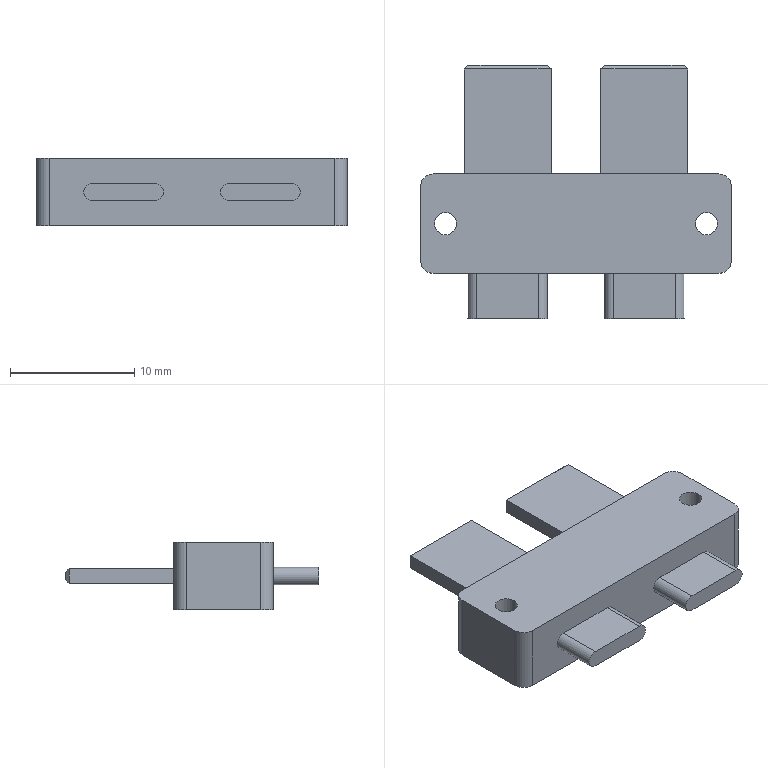Part | SolidWorks | features ICE 2, Chamfer 1, Extrusion 1, Fillet 1 | 1 solid | 42 faces | box 25 x 20.4 x 5.4 mm | volume 1256 mm3 | plane 30 | cylinder 12 | commonest cylinder face diameters 1.4 x4 1.8 x4 2 x4
STEP:
#1=CARTESIAN_POINT('',(-11.4,0.,5.4));
#2=VERTEX_POINT('',#1);
#3=CARTESIAN_POINT('',(-9.6,0.,5.4));
#4=VERTEX_POINT('',#3);
#5=CARTESIAN_POINT('',(-10.5,0.,5.4));
#6=DIRECTION('',(0.,0.,1.));
#7=DIRECTION('',(-1.,0.,0.));
#8=AXIS2_PLACEMENT_3D('',#5,#6,#7);
#9=CIRCLE('',#8,0.9);
#10=EDGE_CURVE('',#2,#4,#9,.T.);
#11=ORIENTED_EDGE('',*,*,#10,.T.);
#12=CARTESIAN_POINT('',(-9.6,0.,0.));
#13=VERTEX_POINT('',#12);
#14=CARTESIAN_POINT('',(-9.6,0.,5.4));
#15=DIRECTION('',(0.,0.,-1.));
#16=VECTOR('',#15,1000.);
#17=LINE('',#14,#16);
#18=EDGE_CURVE('',#4,#13,#17,.T.);
#19=ORIENTED_EDGE('',*,*,#18,.T.);
#20=CARTESIAN_POINT('',(-11.4,0.,0.));
#21=VERTEX_POINT('',#20);
#22=CARTESIAN_POINT('',(-10.5,0.,0.));
#23=DIRECTION('',(0.,0.,1.));
#24=DIRECTION('',(-1.,0.,0.));
#25=AXIS2_PLACEMENT_3D('',#22,#23,#24);
#26=CIRCLE('',#25,0.9);
#27=EDGE_CURVE('',#21,#13,#26,.T.);
#28=ORIENTED_EDGE('',*,*,#27,.F.);
#29=CARTESIAN_POINT('',(-11.4,0.,5.4));
#30=DIRECTION('',(0.,0.,-1.));
#31=VECTOR('',#30,1000.);
#32=LINE('',#29,#31);
#33=EDGE_CURVE('',#2,#21,#32,.T.);
#34=ORIENTED_EDGE('',*,*,#33,.F.);
#35=EDGE_LOOP('',(#11,#19,#28,#34));
#36=FACE_OUTER_BOUND('',#35,.T.);
#37=CARTESIAN_POINT('',(-10.5,0.,5.4));
#38=DIRECTION('',(0.,0.,-1.));
#39=DIRECTION('',(-1.,0.,0.));
#40=AXIS2_PLACEMENT_3D('',#37,#38,#39);
#41=CYLINDRICAL_SURFACE('',#40,0.9);
#42=ADVANCED_FACE('',(#36),#41,.F.);
#43=CARTESIAN_POINT('',(9.6,0.,5.4));
#44=VERTEX_POINT('',#43);
#45=CARTESIAN_POINT('',(11.4,0.,5.4));
#46=VERTEX_POINT('',#45);
#47=CARTESIAN_POINT('',(10.5,0.,5.4));
#48=DIRECTION('',(0.,0.,1.));
#49=DIRECTION('',(1.,0.,0.));
#50=AXIS2_PLACEMENT_3D('',#47,#48,#49);
#51=CIRCLE('',#50,0.9);
#52=EDGE_CURVE('',#44,#46,#51,.T.);
#53=ORIENTED_EDGE('',*,*,#52,.T.);
#54=CARTESIAN_POINT('',(11.4,0.,0.));
#55=VERTEX_POINT('',#54);
#56=CARTESIAN_POINT('',(11.4,0.,5.4));
#57=DIRECTION('',(0.,0.,-1.));
#58=VECTOR('',#57,1000.);
#59=LINE('',#56,#58);
#60=EDGE_CURVE('',#46,#55,#59,.T.);
#61=ORIENTED_EDGE('',*,*,#60,.T.);
#62=CARTESIAN_POINT('',(9.6,0.,0.));
#63=VERTEX_POINT('',#62);
#64=CARTESIAN_POINT('',(10.5,0.,0.));
#65=DIRECTION('',(0.,0.,1.));
#66=DIRECTION('',(1.,0.,0.));
#67=AXIS2_PLACEMENT_3D('',#64,#65,#66);
#68=CIRCLE('',#67,0.9);
#69=EDGE_CURVE('',#63,#55,#68,.T.);
#70=ORIENTED_EDGE('',*,*,#69,.F.);
#71=CARTESIAN_POINT('',(9.6,0.,5.4));
#72=DIRECTION('',(0.,0.,-1.));
#73=VECTOR('',#72,1000.);
#74=LINE('',#71,#73);
#75=EDGE_CURVE('',#44,#63,#74,.T.);
#76=ORIENTED_EDGE('',*,*,#75,.F.);
#77=EDGE_LOOP('',(#53,#61,#70,#76));
#78=FACE_OUTER_BOUND('',#77,.T.);
#79=CARTESIAN_POINT('',(10.5,0.,5.4));
#80=DIRECTION('',(0.,0.,-1.));
#81=DIRECTION('',(-1.,0.,0.));
#82=AXIS2_PLACEMENT_3D('',#79,#80,#81);
#83=CYLINDRICAL_SURFACE('',#82,0.9);
#84=ADVANCED_FACE('',(#78),#83,.F.);
#85=CARTESIAN_POINT('',(9.,4.,3.3));
#86=VERTEX_POINT('',#85);
#87=CARTESIAN_POINT('',(9.,4.,2.1));
#88=VERTEX_POINT('',#87);
#89=CARTESIAN_POINT('',(9.,4.,2.1));
#90=DIRECTION('',(0.,0.,-1.));
#91=VECTOR('',#90,1000.);
#92=LINE('',#89,#91);
#93=EDGE_CURVE('',#86,#88,#92,.T.);
#94=ORIENTED_EDGE('',*,*,#93,.F.);
#95=CARTESIAN_POINT('',(2.,4.,3.3));
#96=VERTEX_POINT('',#95);
#97=CARTESIAN_POINT('',(2.,4.,3.3));
#98=DIRECTION('',(1.,0.,0.));
#99=VECTOR('',#98,1000.);
#100=LINE('',#97,#99);
#101=EDGE_CURVE('',#96,#86,#100,.T.);
#102=ORIENTED_EDGE('',*,*,#101,.F.);
#103=CARTESIAN_POINT('',(2.,4.,2.1));
#104=VERTEX_POINT('',#103);
#105=CARTESIAN_POINT('',(2.,4.,2.1));
#106=DIRECTION('',(0.,0.,1.));
#107=VECTOR('',#106,1000.);
#108=LINE('',#105,#107);
#109=EDGE_CURVE('',#104,#96,#108,.T.);
#110=ORIENTED_EDGE('',*,*,#109,.F.);
#111=CARTESIAN_POINT('',(2.,4.,2.1));
#112=DIRECTION('',(-1.,0.,0.));
#113=VECTOR('',#112,1000.);
#114=LINE('',#111,#113);
#115=EDGE_CURVE('',#88,#104,#114,.T.);
#116=ORIENTED_EDGE('',*,*,#115,.F.);
#117=EDGE_LOOP('',(#94,#102,#110,#116));
#118=FACE_BOUND('',#117,.T.);
#119=CARTESIAN_POINT('',(11.5,4.,5.4));
#120=VERTEX_POINT('',#119);
#121=CARTESIAN_POINT('',(-11.5,4.,5.4));
#122=VERTEX_POINT('',#121);
#123=CARTESIAN_POINT('',(-12.5,4.,5.4));
#124=DIRECTION('',(-1.,0.,0.));
#125=VECTOR('',#124,1000.);
#126=LINE('',#123,#125);
#127=EDGE_CURVE('',#120,#122,#126,.T.);
#128=ORIENTED_EDGE('',*,*,#127,.F.);
#129=CARTESIAN_POINT('',(11.5,4.,0.));
#130=VERTEX_POINT('',#129);
#131=CARTESIAN_POINT('',(11.5,4.,5.4));
#132=DIRECTION('',(0.,0.,-1.));
#133=VECTOR('',#132,1000.);
#134=LINE('',#131,#133);
#135=EDGE_CURVE('',#120,#130,#134,.T.);
#136=ORIENTED_EDGE('',*,*,#135,.T.);
#137=CARTESIAN_POINT('',(-11.5,4.,0.));
#138=VERTEX_POINT('',#137);
#139=CARTESIAN_POINT('',(-12.5,4.,0.));
#140=DIRECTION('',(-1.,0.,0.));
#141=VECTOR('',#140,1000.);
#142=LINE('',#139,#141);
#143=EDGE_CURVE('',#130,#138,#142,.T.);
#144=ORIENTED_EDGE('',*,*,#143,.T.);
#145=CARTESIAN_POINT('',(-11.5,4.,5.4));
#146=DIRECTION('',(0.,0.,1.));
#147=VECTOR('',#146,1000.);
#148=LINE('',#145,#147);
#149=EDGE_CURVE('',#138,#122,#148,.T.);
#150=ORIENTED_EDGE('',*,*,#149,.T.);
#151=EDGE_LOOP('',(#128,#136,#144,#150));
#152=FACE_OUTER_BOUND('',#151,.T.);
#153=CARTESIAN_POINT('',(-2.,4.,3.3));
#154=VERTEX_POINT('',#153);
#155=CARTESIAN_POINT('',(-2.,4.,2.1));
#156=VERTEX_POINT('',#155);
#157=CARTESIAN_POINT('',(-2.,4.,2.1));
#158=DIRECTION('',(0.,0.,-1.));
#159=VECTOR('',#158,1000.);
#160=LINE('',#157,#159);
#161=EDGE_CURVE('',#154,#156,#160,.T.);
#162=ORIENTED_EDGE('',*,*,#161,.F.);
#163=CARTESIAN_POINT('',(-9.,4.,3.3));
#164=VERTEX_POINT('',#163);
#165=CARTESIAN_POINT('',(-2.,4.,3.3));
#166=DIRECTION('',(1.,0.,0.));
#167=VECTOR('',#166,1000.);
#168=LINE('',#165,#167);
#169=EDGE_CURVE('',#164,#154,#168,.T.);
#170=ORIENTED_EDGE('',*,*,#169,.F.);
#171=CARTESIAN_POINT('',(-9.,4.,2.1));
#172=VERTEX_POINT('',#171);
#173=CARTESIAN_POINT('',(-9.,4.,2.1));
#174=DIRECTION('',(0.,0.,1.));
#175=VECTOR('',#174,1000.);
#176=LINE('',#173,#175);
#177=EDGE_CURVE('',#172,#164,#176,.T.);
#178=ORIENTED_EDGE('',*,*,#177,.F.);
#179=CARTESIAN_POINT('',(-2.,4.,2.1));
#180=DIRECTION('',(-1.,0.,0.));
#181=VECTOR('',#180,1000.);
#182=LINE('',#179,#181);
#183=EDGE_CURVE('',#156,#172,#182,.T.);
#184=ORIENTED_EDGE('',*,*,#183,.F.);
#185=EDGE_LOOP('',(#162,#170,#178,#184));
#186=FACE_BOUND('',#185,.T.);
#187=CARTESIAN_POINT('',(-12.5,4.,5.4));
#188=DIRECTION('',(0.,-1.,0.));
#189=DIRECTION('',(0.,0.,-1.));
#190=AXIS2_PLACEMENT_3D('',#187,#188,#189);
#191=PLANE('',#190);
#192=ADVANCED_FACE('',(#118,#152,#186),#191,.F.);
#193=CARTESIAN_POINT('',(3.,-4.,3.4));
#194=VERTEX_POINT('',#193);
#195=CARTESIAN_POINT('',(3.,-4.,2.));
#196=VERTEX_POINT('',#195);
#197=CARTESIAN_POINT('',(3.,-4.,2.7));
#198=DIRECTION('',(0.,-1.,0.));
#199=DIRECTION('',(0.,0.,-1.));
#200=AXIS2_PLACEMENT_3D('',#197,#198,#199);
#201=CIRCLE('',#200,0.7);
#202=EDGE_CURVE('',#194,#196,#201,.T.);
#203=ORIENTED_EDGE('',*,*,#202,.F.);
#204=CARTESIAN_POINT('',(8.,-4.,3.4));
#205=VERTEX_POINT('',#204);
#206=CARTESIAN_POINT('',(3.,-4.,3.4));
#207=DIRECTION('',(-1.,0.,0.));
#208=VECTOR('',#207,1000.);
#209=LINE('',#206,#208);
#210=EDGE_CURVE('',#205,#194,#209,.T.);
#211=ORIENTED_EDGE('',*,*,#210,.F.);
#212=CARTESIAN_POINT('',(8.,-4.,2.));
#213=VERTEX_POINT('',#212);
#214=CARTESIAN_POINT('',(8.,-4.,2.7));
#215=DIRECTION('',(0.,-1.,0.));
#216=DIRECTION('',(0.,0.,-1.));
#217=AXIS2_PLACEMENT_3D('',#214,#215,#216);
#218=CIRCLE('',#217,0.7);
#219=EDGE_CURVE('',#213,#205,#218,.T.);
#220=ORIENTED_EDGE('',*,*,#219,.F.);
#221=CARTESIAN_POINT('',(3.,-4.,2.));
#222=DIRECTION('',(1.,0.,0.));
#223=VECTOR('',#222,1000.);
#224=LINE('',#221,#223);
#225=EDGE_CURVE('',#196,#213,#224,.T.);
#226=ORIENTED_EDGE('',*,*,#225,.F.);
#227=EDGE_LOOP('',(#203,#211,#220,#226));
#228=FACE_BOUND('',#227,.T.);
#229=CARTESIAN_POINT('',(-11.5,-4.,0.));
#230=VERTEX_POINT('',#229);
#231=CARTESIAN_POINT('',(11.5,-4.,0.));
#232=VERTEX_POINT('',#231);
#233=CARTESIAN_POINT('',(-12.5,-4.,0.));
#234=DIRECTION('',(1.,0.,0.));
#235=VECTOR('',#234,1000.);
#236=LINE('',#233,#235);
#237=EDGE_CURVE('',#230,#232,#236,.T.);
#238=ORIENTED_EDGE('',*,*,#237,.T.);
#239=CARTESIAN_POINT('',(11.5,-4.,5.4));
#240=VERTEX_POINT('',#239);
#241=CARTESIAN_POINT('',(11.5,-4.,5.4));
#242=DIRECTION('',(0.,0.,1.));
#243=VECTOR('',#242,1000.);
#244=LINE('',#241,#243);
#245=EDGE_CURVE('',#232,#240,#244,.T.);
#246=ORIENTED_EDGE('',*,*,#245,.T.);
#247=CARTESIAN_POINT('',(-11.5,-4.,5.4));
#248=VERTEX_POINT('',#247);
#249=CARTESIAN_POINT('',(-12.5,-4.,5.4));
#250=DIRECTION('',(1.,0.,0.));
#251=VECTOR('',#250,1000.);
#252=LINE('',#249,#251);
#253=EDGE_CURVE('',#248,#240,#252,.T.);
#254=ORIENTED_EDGE('',*,*,#253,.F.);
#255=CARTESIAN_POINT('',(-11.5,-4.,5.4));
#256=DIRECTION('',(0.,0.,-1.));
#257=VECTOR('',#256,1000.);
#258=LINE('',#255,#257);
#259=EDGE_CURVE('',#248,#230,#258,.T.);
#260=ORIENTED_EDGE('',*,*,#259,.T.);
#261=EDGE_LOOP('',(#238,#246,#254,#260));
#262=FACE_OUTER_BOUND('',#261,.T.);
#263=CARTESIAN_POINT('',(-3.,-4.,2.));
#264=VERTEX_POINT('',#263);
#265=CARTESIAN_POINT('',(-3.,-4.,3.4));
#266=VERTEX_POINT('',#265);
#267=CARTESIAN_POINT('',(-3.,-4.,2.7));
#268=DIRECTION('',(0.,-1.,0.));
#269=DIRECTION('',(0.,0.,1.));
#270=AXIS2_PLACEMENT_3D('',#267,#268,#269);
#271=CIRCLE('',#270,0.7);
#272=EDGE_CURVE('',#264,#266,#271,.T.);
#273=ORIENTED_EDGE('',*,*,#272,.F.);
#274=CARTESIAN_POINT('',(-8.,-4.,2.));
#275=VERTEX_POINT('',#274);
#276=CARTESIAN_POINT('',(-3.,-4.,2.));
#277=DIRECTION('',(1.,0.,0.));
#278=VECTOR('',#277,1000.);
#279=LINE('',#276,#278);
#280=EDGE_CURVE('',#275,#264,#279,.T.);
#281=ORIENTED_EDGE('',*,*,#280,.F.);
#282=CARTESIAN_POINT('',(-8.,-4.,3.4));
#283=VERTEX_POINT('',#282);
#284=CARTESIAN_POINT('',(-8.,-4.,2.7));
#285=DIRECTION('',(0.,-1.,0.));
#286=DIRECTION('',(0.,0.,1.));
#287=AXIS2_PLACEMENT_3D('',#284,#285,#286);
#288=CIRCLE('',#287,0.7);
#289=EDGE_CURVE('',#283,#275,#288,.T.);
#290=ORIENTED_EDGE('',*,*,#289,.F.);
#291=CARTESIAN_POINT('',(-3.,-4.,3.4));
#292=DIRECTION('',(-1.,0.,0.));
#293=VECTOR('',#292,1000.);
#294=LINE('',#291,#293);
#295=EDGE_CURVE('',#266,#283,#294,.T.);
#296=ORIENTED_EDGE('',*,*,#295,.F.);
#297=EDGE_LOOP('',(#273,#281,#290,#296));
#298=FACE_BOUND('',#297,.T.);
#299=CARTESIAN_POINT('',(-12.5,-4.,5.4));
#300=DIRECTION('',(0.,1.,0.));
#301=DIRECTION('',(0.,0.,1.));
#302=AXIS2_PLACEMENT_3D('',#299,#300,#301);
#303=PLANE('',#302);
#304=ADVANCED_FACE('',(#228,#262,#298),#303,.F.);
#305=ORIENTED_EDGE('',*,*,#52,.F.);
#306=CARTESIAN_POINT('',(10.5,0.,5.4));
#307=DIRECTION('',(0.,0.,1.));
#308=DIRECTION('',(1.,0.,0.));
#309=AXIS2_PLACEMENT_3D('',#306,#307,#308);
#310=CIRCLE('',#309,0.9);
#311=EDGE_CURVE('',#46,#44,#310,.T.);
#312=ORIENTED_EDGE('',*,*,#311,.F.);
#313=EDGE_LOOP('',(#305,#312));
#314=FACE_BOUND('',#313,.T.);
#315=ORIENTED_EDGE('',*,*,#253,.T.);
#316=CARTESIAN_POINT('',(12.5,-3.,5.4));
#317=VERTEX_POINT('',#316);
#318=CARTESIAN_POINT('',(11.5,-3.,5.4));
#319=DIRECTION('',(0.,0.,1.));
#320=DIRECTION('',(1.,0.,0.));
#321=AXIS2_PLACEMENT_3D('',#318,#319,#320);
#322=CIRCLE('',#321,1.);
#323=EDGE_CURVE('',#240,#317,#322,.T.);
#324=ORIENTED_EDGE('',*,*,#323,.T.);
#325=CARTESIAN_POINT('',(12.5,3.,5.4));
#326=VERTEX_POINT('',#325);
#327=CARTESIAN_POINT('',(12.5,4.,5.4));
#328=DIRECTION('',(0.,1.,0.));
#329=VECTOR('',#328,1000.);
#330=LINE('',#327,#329);
#331=EDGE_CURVE('',#317,#326,#330,.T.);
#332=ORIENTED_EDGE('',*,*,#331,.T.);
#333=CARTESIAN_POINT('',(11.5,3.,5.4));
#334=DIRECTION('',(0.,0.,1.));
#335=DIRECTION('',(1.,0.,0.));
#336=AXIS2_PLACEMENT_3D('',#333,#334,#335);
#337=CIRCLE('',#336,1.);
#338=EDGE_CURVE('',#326,#120,#337,.T.);
#339=ORIENTED_EDGE('',*,*,#338,.T.);
#340=ORIENTED_EDGE('',*,*,#127,.T.);
#341=CARTESIAN_POINT('',(-12.5,3.,5.4));
#342=VERTEX_POINT('',#341);
#343=CARTESIAN_POINT('',(-11.5,3.,5.4));
#344=DIRECTION('',(0.,0.,1.));
#345=DIRECTION('',(1.,0.,0.));
#346=AXIS2_PLACEMENT_3D('',#343,#344,#345);
#347=CIRCLE('',#346,1.);
#348=EDGE_CURVE('',#122,#342,#347,.T.);
#349=ORIENTED_EDGE('',*,*,#348,.T.);
#350=CARTESIAN_POINT('',(-12.5,-3.,5.4));
#351=VERTEX_POINT('',#350);
#352=CARTESIAN_POINT('',(-12.5,4.,5.4));
#353=DIRECTION('',(0.,-1.,0.));
#354=VECTOR('',#353,1000.);
#355=LINE('',#352,#354);
#356=EDGE_CURVE('',#342,#351,#355,.T.);
#357=ORIENTED_EDGE('',*,*,#356,.T.);
#358=CARTESIAN_POINT('',(-11.5,-3.,5.4));
#359=DIRECTION('',(0.,0.,1.));
#360=DIRECTION('',(1.,0.,0.));
#361=AXIS2_PLACEMENT_3D('',#358,#359,#360);
#362=CIRCLE('',#361,1.);
#363=EDGE_CURVE('',#351,#248,#362,.T.);
#364=ORIENTED_EDGE('',*,*,#363,.T.);
#365=EDGE_LOOP('',(#315,#324,#332,#339,#340,#349,#357,#364));
#366=FACE_OUTER_BOUND('',#365,.T.);
#367=ORIENTED_EDGE('',*,*,#10,.F.);
#368=CARTESIAN_POINT('',(-10.5,0.,5.4));
#369=DIRECTION('',(0.,0.,1.));
#370=DIRECTION('',(-1.,0.,0.));
#371=AXIS2_PLACEMENT_3D('',#368,#369,#370);
#372=CIRCLE('',#371,0.9);
#373=EDGE_CURVE('',#4,#2,#372,.T.);
#374=ORIENTED_EDGE('',*,*,#373,.F.);
#375=EDGE_LOOP('',(#367,#374));
#376=FACE_BOUND('',#375,.T.);
#377=CARTESIAN_POINT('',(0.,0.,5.4));
#378=DIRECTION('',(0.,0.,1.));
#379=DIRECTION('',(1.,0.,0.));
#380=AXIS2_PLACEMENT_3D('',#377,#378,#379);
#381=PLANE('',#380);
#382=ADVANCED_FACE('',(#314,#366,#376),#381,.T.);
#383=CARTESIAN_POINT('',(12.5,-3.,0.));
#384=VERTEX_POINT('',#383);
#385=CARTESIAN_POINT('',(12.5,3.,0.));
#386=VERTEX_POINT('',#385);
#387=CARTESIAN_POINT('',(12.5,4.,0.));
#388=DIRECTION('',(0.,1.,0.));
#389=VECTOR('',#388,1000.);
#390=LINE('',#387,#389);
#391=EDGE_CURVE('',#384,#386,#390,.T.);
#392=ORIENTED_EDGE('',*,*,#391,.F.);
#393=CARTESIAN_POINT('',(11.5,-3.,0.));
#394=DIRECTION('',(0.,0.,-1.));
#395=DIRECTION('',(1.,0.,0.));
#396=AXIS2_PLACEMENT_3D('',#393,#394,#395);
#397=CIRCLE('',#396,1.);
#398=EDGE_CURVE('',#384,#232,#397,.T.);
#399=ORIENTED_EDGE('',*,*,#398,.T.);
#400=ORIENTED_EDGE('',*,*,#237,.F.);
#401=CARTESIAN_POINT('',(-12.5,-3.,0.));
#402=VERTEX_POINT('',#401);
#403=CARTESIAN_POINT('',(-11.5,-3.,0.));
#404=DIRECTION('',(0.,0.,-1.));
#405=DIRECTION('',(1.,0.,0.));
#406=AXIS2_PLACEMENT_3D('',#403,#404,#405);
#407=CIRCLE('',#406,1.);
#408=EDGE_CURVE('',#230,#402,#407,.T.);
#409=ORIENTED_EDGE('',*,*,#408,.T.);
#410=CARTESIAN_POINT('',(-12.5,3.,0.));
#411=VERTEX_POINT('',#410);
#412=CARTESIAN_POINT('',(-12.5,4.,0.));
#413=DIRECTION('',(0.,-1.,0.));
#414=VECTOR('',#413,1000.);
#415=LINE('',#412,#414);
#416=EDGE_CURVE('',#411,#402,#415,.T.);
#417=ORIENTED_EDGE('',*,*,#416,.F.);
#418=CARTESIAN_POINT('',(-11.5,3.,0.));
#419=DIRECTION('',(0.,0.,-1.));
#420=DIRECTION('',(1.,0.,0.));
#421=AXIS2_PLACEMENT_3D('',#418,#419,#420);
#422=CIRCLE('',#421,1.);
#423=EDGE_CURVE('',#411,#138,#422,.T.);
#424=ORIENTED_EDGE('',*,*,#423,.T.);
#425=ORIENTED_EDGE('',*,*,#143,.F.);
#426=CARTESIAN_POINT('',(11.5,3.,0.));
#427=DIRECTION('',(0.,0.,-1.));
#428=DIRECTION('',(1.,0.,0.));
#429=AXIS2_PLACEMENT_3D('',#426,#427,#428);
#430=CIRCLE('',#429,1.);
#431=EDGE_CURVE('',#130,#386,#430,.T.);
#432=ORIENTED_EDGE('',*,*,#431,.T.);
#433=EDGE_LOOP('',(#392,#399,#400,#409,#417,#424,#425,#432));
#434=FACE_OUTER_BOUND('',#433,.T.);
#435=ORIENTED_EDGE('',*,*,#69,.T.);
#436=CARTESIAN_POINT('',(10.5,0.,0.));
#437=DIRECTION('',(0.,0.,1.));
#438=DIRECTION('',(1.,0.,0.));
#439=AXIS2_PLACEMENT_3D('',#436,#437,#438);
#440=CIRCLE('',#439,0.9);
#441=EDGE_CURVE('',#55,#63,#440,.T.);
#442=ORIENTED_EDGE('',*,*,#441,.T.);
#443=EDGE_LOOP('',(#435,#442));
#444=FACE_BOUND('',#443,.T.);
#445=ORIENTED_EDGE('',*,*,#27,.T.);
#446=CARTESIAN_POINT('',(-10.5,0.,0.));
#447=DIRECTION('',(0.,0.,1.));
#448=DIRECTION('',(-1.,0.,0.));
#449=AXIS2_PLACEMENT_3D('',#446,#447,#448);
#450=CIRCLE('',#449,0.9);
#451=EDGE_CURVE('',#13,#21,#450,.T.);
#452=ORIENTED_EDGE('',*,*,#451,.T.);
#453=EDGE_LOOP('',(#445,#452));
#454=FACE_BOUND('',#453,.T.);
#455=CARTESIAN_POINT('',(0.,0.,0.));
#456=DIRECTION('',(0.,0.,1.));
#457=DIRECTION('',(1.,0.,0.));
#458=AXIS2_PLACEMENT_3D('',#455,#456,#457);
#459=PLANE('',#458);
#460=ADVANCED_FACE('',(#434,#444,#454),#459,.F.);
#461=ORIENTED_EDGE('',*,*,#331,.F.);
#462=CARTESIAN_POINT('',(12.5,-3.,5.4));
#463=DIRECTION('',(0.,0.,-1.));
#464=VECTOR('',#463,1000.);
#465=LINE('',#462,#464);
#466=EDGE_CURVE('',#317,#384,#465,.T.);
#467=ORIENTED_EDGE('',*,*,#466,.T.);
#468=ORIENTED_EDGE('',*,*,#391,.T.);
#469=CARTESIAN_POINT('',(12.5,3.,5.4));
#470=DIRECTION('',(0.,0.,1.));
#471=VECTOR('',#470,1000.);
#472=LINE('',#469,#471);
#473=EDGE_CURVE('',#386,#326,#472,.T.);
#474=ORIENTED_EDGE('',*,*,#473,.T.);
#475=EDGE_LOOP('',(#461,#467,#468,#474));
#476=FACE_OUTER_BOUND('',#475,.T.);
#477=CARTESIAN_POINT('',(12.5,4.,5.4));
#478=DIRECTION('',(-1.,0.,0.));
#479=DIRECTION('',(0.,0.,1.));
#480=AXIS2_PLACEMENT_3D('',#477,#478,#479);
#481=PLANE('',#480);
#482=ADVANCED_FACE('',(#476),#481,.F.);
#483=ORIENTED_EDGE('',*,*,#416,.T.);
#484=CARTESIAN_POINT('',(-12.5,-3.,5.4));
#485=DIRECTION('',(0.,0.,1.));
#486=VECTOR('',#485,1000.);
#487=LINE('',#484,#486);
#488=EDGE_CURVE('',#402,#351,#487,.T.);
#489=ORIENTED_EDGE('',*,*,#488,.T.);
#490=ORIENTED_EDGE('',*,*,#356,.F.);
#491=CARTESIAN_POINT('',(-12.5,3.,5.4));
#492=DIRECTION('',(0.,0.,-1.));
#493=VECTOR('',#492,1000.);
#494=LINE('',#491,#493);
#495=EDGE_CURVE('',#342,#411,#494,.T.);
#496=ORIENTED_EDGE('',*,*,#495,.T.);
#497=EDGE_LOOP('',(#483,#489,#490,#496));
#498=FACE_OUTER_BOUND('',#497,.T.);
#499=CARTESIAN_POINT('',(-12.5,4.,5.4));
#500=DIRECTION('',(1.,0.,0.));
#501=DIRECTION('',(0.,1.,0.));
#502=AXIS2_PLACEMENT_3D('',#499,#500,#501);
#503=PLANE('',#502);
#504=ADVANCED_FACE('',(#498),#503,.F.);
#505=ORIENTED_EDGE('',*,*,#60,.F.);
#506=ORIENTED_EDGE('',*,*,#311,.T.);
#507=ORIENTED_EDGE('',*,*,#75,.T.);
#508=ORIENTED_EDGE('',*,*,#441,.F.);
#509=EDGE_LOOP('',(#505,#506,#507,#508));
#510=FACE_OUTER_BOUND('',#509,.T.);
#511=CARTESIAN_POINT('',(10.5,0.,5.4));
#512=DIRECTION('',(0.,0.,-1.));
#513=DIRECTION('',(-1.,0.,0.));
#514=AXIS2_PLACEMENT_3D('',#511,#512,#513);
#515=CYLINDRICAL_SURFACE('',#514,0.9);
#516=ADVANCED_FACE('',(#510),#515,.F.);
#517=ORIENTED_EDGE('',*,*,#18,.F.);
#518=ORIENTED_EDGE('',*,*,#373,.T.);
#519=ORIENTED_EDGE('',*,*,#33,.T.);
#520=ORIENTED_EDGE('',*,*,#451,.F.);
#521=EDGE_LOOP('',(#517,#518,#519,#520));
#522=FACE_OUTER_BOUND('',#521,.T.);
#523=CARTESIAN_POINT('',(-10.5,0.,5.4));
#524=DIRECTION('',(0.,0.,-1.));
#525=DIRECTION('',(-1.,0.,0.));
#526=AXIS2_PLACEMENT_3D('',#523,#524,#525);
#527=CYLINDRICAL_SURFACE('',#526,0.9);
#528=ADVANCED_FACE('',(#522),#527,.F.);
#529=ORIENTED_EDGE('',*,*,#202,.T.);
#530=CARTESIAN_POINT('',(3.,-7.65,2.));
#531=VERTEX_POINT('',#530);
#532=CARTESIAN_POINT('',(3.,-7.65,2.));
#533=DIRECTION('',(0.,1.,0.));
#534=VECTOR('',#533,1000.);
#535=LINE('',#532,#534);
#536=EDGE_CURVE('',#531,#196,#535,.T.);
#537=ORIENTED_EDGE('',*,*,#536,.F.);
#538=CARTESIAN_POINT('',(3.,-7.65,3.4));
#539=VERTEX_POINT('',#538);
#540=CARTESIAN_POINT('',(3.,-7.65,2.7));
#541=DIRECTION('',(0.,-1.,0.));
#542=DIRECTION('',(0.,0.,-1.));
#543=AXIS2_PLACEMENT_3D('',#540,#541,#542);
#544=CIRCLE('',#543,0.7);
#545=EDGE_CURVE('',#539,#531,#544,.T.);
#546=ORIENTED_EDGE('',*,*,#545,.F.);
#547=CARTESIAN_POINT('',(3.,-7.65,3.4));
#548=DIRECTION('',(0.,1.,0.));
#549=VECTOR('',#548,1000.);
#550=LINE('',#547,#549);
#551=EDGE_CURVE('',#539,#194,#550,.T.);
#552=ORIENTED_EDGE('',*,*,#551,.T.);
#553=EDGE_LOOP('',(#529,#537,#546,#552));
#554=FACE_OUTER_BOUND('',#553,.T.);
#555=CARTESIAN_POINT('',(3.,-7.65,2.7));
#556=DIRECTION('',(0.,1.,0.));
#557=DIRECTION('',(0.,0.,1.));
#558=AXIS2_PLACEMENT_3D('',#555,#556,#557);
#559=CYLINDRICAL_SURFACE('',#558,0.7);
#560=ADVANCED_FACE('',(#554),#559,.T.);
#561=ORIENTED_EDGE('',*,*,#225,.T.);
#562=CARTESIAN_POINT('',(8.,-7.65,2.));
#563=VERTEX_POINT('',#562);
#564=CARTESIAN_POINT('',(8.,-7.65,2.));
#565=DIRECTION('',(0.,1.,0.));
#566=VECTOR('',#565,1000.);
#567=LINE('',#564,#566);
#568=EDGE_CURVE('',#563,#213,#567,.T.);
#569=ORIENTED_EDGE('',*,*,#568,.F.);
#570=CARTESIAN_POINT('',(3.,-7.65,2.));
#571=DIRECTION('',(1.,0.,0.));
#572=VECTOR('',#571,1000.);
#573=LINE('',#570,#572);
#574=EDGE_CURVE('',#531,#563,#573,.T.);
#575=ORIENTED_EDGE('',*,*,#574,.F.);
#576=ORIENTED_EDGE('',*,*,#536,.T.);
#577=EDGE_LOOP('',(#561,#569,#575,#576));
#578=FACE_OUTER_BOUND('',#577,.T.);
#579=CARTESIAN_POINT('',(3.,-7.65,2.));
#580=DIRECTION('',(0.,0.,1.));
#581=DIRECTION('',(1.,0.,0.));
#582=AXIS2_PLACEMENT_3D('',#579,#580,#581);
#583=PLANE('',#582);
#584=ADVANCED_FACE('',(#578),#583,.F.);
#585=ORIENTED_EDGE('',*,*,#219,.T.);
#586=CARTESIAN_POINT('',(8.,-7.65,3.4));
#587=VERTEX_POINT('',#586);
#588=CARTESIAN_POINT('',(8.,-7.65,3.4));
#589=DIRECTION('',(0.,1.,0.));
#590=VECTOR('',#589,1000.);
#591=LINE('',#588,#590);
#592=EDGE_CURVE('',#587,#205,#591,.T.);
#593=ORIENTED_EDGE('',*,*,#592,.F.);
#594=CARTESIAN_POINT('',(8.,-7.65,2.7));
#595=DIRECTION('',(0.,-1.,0.));
#596=DIRECTION('',(0.,0.,-1.));
#597=AXIS2_PLACEMENT_3D('',#594,#595,#596);
#598=CIRCLE('',#597,0.7);
#599=EDGE_CURVE('',#563,#587,#598,.T.);
#600=ORIENTED_EDGE('',*,*,#599,.F.);
#601=ORIENTED_EDGE('',*,*,#568,.T.);
#602=EDGE_LOOP('',(#585,#593,#600,#601));
#603=FACE_OUTER_BOUND('',#602,.T.);
#604=CARTESIAN_POINT('',(8.,-7.65,2.7));
#605=DIRECTION('',(0.,1.,0.));
#606=DIRECTION('',(0.,0.,1.));
#607=AXIS2_PLACEMENT_3D('',#604,#605,#606);
#608=CYLINDRICAL_SURFACE('',#607,0.7);
#609=ADVANCED_FACE('',(#603),#608,.T.);
#610=ORIENTED_EDGE('',*,*,#210,.T.);
#611=ORIENTED_EDGE('',*,*,#551,.F.);
#612=CARTESIAN_POINT('',(3.,-7.65,3.4));
#613=DIRECTION('',(-1.,0.,0.));
#614=VECTOR('',#613,1000.);
#615=LINE('',#612,#614);
#616=EDGE_CURVE('',#587,#539,#615,.T.);
#617=ORIENTED_EDGE('',*,*,#616,.F.);
#618=ORIENTED_EDGE('',*,*,#592,.T.);
#619=EDGE_LOOP('',(#610,#611,#617,#618));
#620=FACE_OUTER_BOUND('',#619,.T.);
#621=CARTESIAN_POINT('',(3.,-7.65,3.4));
#622=DIRECTION('',(0.,0.,-1.));
#623=DIRECTION('',(-1.,0.,0.));
#624=AXIS2_PLACEMENT_3D('',#621,#622,#623);
#625=PLANE('',#624);
#626=ADVANCED_FACE('',(#620),#625,.F.);
#627=ORIENTED_EDGE('',*,*,#545,.T.);
#628=ORIENTED_EDGE('',*,*,#574,.T.);
#629=ORIENTED_EDGE('',*,*,#599,.T.);
#630=ORIENTED_EDGE('',*,*,#616,.T.);
#631=EDGE_LOOP('',(#627,#628,#629,#630));
#632=FACE_OUTER_BOUND('',#631,.T.);
#633=CARTESIAN_POINT('',(3.,-7.65,2.7));
#634=DIRECTION('',(0.,-1.,0.));
#635=DIRECTION('',(0.,0.,-1.));
#636=AXIS2_PLACEMENT_3D('',#633,#634,#635);
#637=PLANE('',#636);
#638=ADVANCED_FACE('',(#632),#637,.T.);
#639=ORIENTED_EDGE('',*,*,#272,.T.);
#640=CARTESIAN_POINT('',(-3.,-7.65,3.4));
#641=VERTEX_POINT('',#640);
#642=CARTESIAN_POINT('',(-3.,-7.65,3.4));
#643=DIRECTION('',(0.,1.,0.));
#644=VECTOR('',#643,1000.);
#645=LINE('',#642,#644);
#646=EDGE_CURVE('',#641,#266,#645,.T.);
#647=ORIENTED_EDGE('',*,*,#646,.F.);
#648=CARTESIAN_POINT('',(-3.,-7.65,2.));
#649=VERTEX_POINT('',#648);
#650=CARTESIAN_POINT('',(-3.,-7.65,2.7));
#651=DIRECTION('',(0.,-1.,0.));
#652=DIRECTION('',(0.,0.,1.));
#653=AXIS2_PLACEMENT_3D('',#650,#651,#652);
#654=CIRCLE('',#653,0.7);
#655=EDGE_CURVE('',#649,#641,#654,.T.);
#656=ORIENTED_EDGE('',*,*,#655,.F.);
#657=CARTESIAN_POINT('',(-3.,-7.65,2.));
#658=DIRECTION('',(0.,1.,0.));
#659=VECTOR('',#658,1000.);
#660=LINE('',#657,#659);
#661=EDGE_CURVE('',#649,#264,#660,.T.);
#662=ORIENTED_EDGE('',*,*,#661,.T.);
#663=EDGE_LOOP('',(#639,#647,#656,#662));
#664=FACE_OUTER_BOUND('',#663,.T.);
#665=CARTESIAN_POINT('',(-3.,-7.65,2.7));
#666=DIRECTION('',(0.,1.,0.));
#667=DIRECTION('',(0.,0.,1.));
#668=AXIS2_PLACEMENT_3D('',#665,#666,#667);
#669=CYLINDRICAL_SURFACE('',#668,0.7);
#670=ADVANCED_FACE('',(#664),#669,.T.);
#671=ORIENTED_EDGE('',*,*,#295,.T.);
#672=CARTESIAN_POINT('',(-8.,-7.65,3.4));
#673=VERTEX_POINT('',#672);
#674=CARTESIAN_POINT('',(-8.,-7.65,3.4));
#675=DIRECTION('',(0.,1.,0.));
#676=VECTOR('',#675,1000.);
#677=LINE('',#674,#676);
#678=EDGE_CURVE('',#673,#283,#677,.T.);
#679=ORIENTED_EDGE('',*,*,#678,.F.);
#680=CARTESIAN_POINT('',(-3.,-7.65,3.4));
#681=DIRECTION('',(-1.,0.,0.));
#682=VECTOR('',#681,1000.);
#683=LINE('',#680,#682);
#684=EDGE_CURVE('',#641,#673,#683,.T.);
#685=ORIENTED_EDGE('',*,*,#684,.F.);
#686=ORIENTED_EDGE('',*,*,#646,.T.);
#687=EDGE_LOOP('',(#671,#679,#685,#686));
#688=FACE_OUTER_BOUND('',#687,.T.);
#689=CARTESIAN_POINT('',(-3.,-7.65,3.4));
#690=DIRECTION('',(0.,0.,-1.));
#691=DIRECTION('',(-1.,0.,0.));
#692=AXIS2_PLACEMENT_3D('',#689,#690,#691);
#693=PLANE('',#692);
#694=ADVANCED_FACE('',(#688),#693,.F.);
#695=ORIENTED_EDGE('',*,*,#289,.T.);
#696=CARTESIAN_POINT('',(-8.,-7.65,2.));
#697=VERTEX_POINT('',#696);
#698=CARTESIAN_POINT('',(-8.,-7.65,2.));
#699=DIRECTION('',(0.,1.,0.));
#700=VECTOR('',#699,1000.);
#701=LINE('',#698,#700);
#702=EDGE_CURVE('',#697,#275,#701,.T.);
#703=ORIENTED_EDGE('',*,*,#702,.F.);
#704=CARTESIAN_POINT('',(-8.,-7.65,2.7));
#705=DIRECTION('',(0.,-1.,0.));
#706=DIRECTION('',(0.,0.,1.));
#707=AXIS2_PLACEMENT_3D('',#704,#705,#706);
#708=CIRCLE('',#707,0.7);
#709=EDGE_CURVE('',#673,#697,#708,.T.);
#710=ORIENTED_EDGE('',*,*,#709,.F.);
#711=ORIENTED_EDGE('',*,*,#678,.T.);
#712=EDGE_LOOP('',(#695,#703,#710,#711));
#713=FACE_OUTER_BOUND('',#712,.T.);
#714=CARTESIAN_POINT('',(-8.,-7.65,2.7));
#715=DIRECTION('',(0.,1.,0.));
#716=DIRECTION('',(0.,0.,1.));
#717=AXIS2_PLACEMENT_3D('',#714,#715,#716);
#718=CYLINDRICAL_SURFACE('',#717,0.7);
#719=ADVANCED_FACE('',(#713),#718,.T.);
#720=ORIENTED_EDGE('',*,*,#280,.T.);
#721=ORIENTED_EDGE('',*,*,#661,.F.);
#722=CARTESIAN_POINT('',(-3.,-7.65,2.));
#723=DIRECTION('',(1.,0.,0.));
#724=VECTOR('',#723,1000.);
#725=LINE('',#722,#724);
#726=EDGE_CURVE('',#697,#649,#725,.T.);
#727=ORIENTED_EDGE('',*,*,#726,.F.);
#728=ORIENTED_EDGE('',*,*,#702,.T.);
#729=EDGE_LOOP('',(#720,#721,#727,#728));
#730=FACE_OUTER_BOUND('',#729,.T.);
#731=CARTESIAN_POINT('',(-3.,-7.65,2.));
#732=DIRECTION('',(0.,0.,1.));
#733=DIRECTION('',(1.,0.,0.));
#734=AXIS2_PLACEMENT_3D('',#731,#732,#733);
#735=PLANE('',#734);
#736=ADVANCED_FACE('',(#730),#735,.F.);
#737=ORIENTED_EDGE('',*,*,#655,.T.);
#738=ORIENTED_EDGE('',*,*,#684,.T.);
#739=ORIENTED_EDGE('',*,*,#709,.T.);
#740=ORIENTED_EDGE('',*,*,#726,.T.);
#741=EDGE_LOOP('',(#737,#738,#739,#740));
#742=FACE_OUTER_BOUND('',#741,.T.);
#743=CARTESIAN_POINT('',(-3.,-7.65,2.7));
#744=DIRECTION('',(0.,1.,0.));
#745=DIRECTION('',(0.,0.,1.));
#746=AXIS2_PLACEMENT_3D('',#743,#744,#745);
#747=PLANE('',#746);
#748=ADVANCED_FACE('',(#742),#747,.F.);
#749=CARTESIAN_POINT('',(9.,12.45,2.1));
#750=VERTEX_POINT('',#749);
#751=CARTESIAN_POINT('',(9.,12.75,2.1));
#752=DIRECTION('',(0.,-1.,0.));
#753=VECTOR('',#752,1000.);
#754=LINE('',#751,#753);
#755=EDGE_CURVE('',#750,#88,#754,.T.);
#756=ORIENTED_EDGE('',*,*,#755,.F.);
#757=CARTESIAN_POINT('',(9.,12.45,3.3));
#758=VERTEX_POINT('',#757);
#759=CARTESIAN_POINT('',(9.,12.45,3.3));
#760=DIRECTION('',(0.,0.,1.));
#761=VECTOR('',#760,1000.);
#762=LINE('',#759,#761);
#763=EDGE_CURVE('',#750,#758,#762,.T.);
#764=ORIENTED_EDGE('',*,*,#763,.T.);
#765=CARTESIAN_POINT('',(9.,12.75,3.3));
#766=DIRECTION('',(0.,-1.,0.));
#767=VECTOR('',#766,1000.);
#768=LINE('',#765,#767);
#769=EDGE_CURVE('',#758,#86,#768,.T.);
#770=ORIENTED_EDGE('',*,*,#769,.T.);
#771=ORIENTED_EDGE('',*,*,#93,.T.);
#772=EDGE_LOOP('',(#756,#764,#770,#771));
#773=FACE_OUTER_BOUND('',#772,.T.);
#774=CARTESIAN_POINT('',(9.,12.75,2.1));
#775=DIRECTION('',(-1.,0.,0.));
#776=DIRECTION('',(0.,0.,1.));
#777=AXIS2_PLACEMENT_3D('',#774,#775,#776);
#778=PLANE('',#777);
#779=ADVANCED_FACE('',(#773),#778,.F.);
#780=CARTESIAN_POINT('',(2.,12.45,2.1));
#781=VERTEX_POINT('',#780);
#782=CARTESIAN_POINT('',(2.,12.75,2.1));
#783=DIRECTION('',(0.,-1.,0.));
#784=VECTOR('',#783,1000.);
#785=LINE('',#782,#784);
#786=EDGE_CURVE('',#781,#104,#785,.T.);
#787=ORIENTED_EDGE('',*,*,#786,.F.);
#788=CARTESIAN_POINT('',(9.,12.45,2.1));
#789=DIRECTION('',(1.,0.,0.));
#790=VECTOR('',#789,1000.);
#791=LINE('',#788,#790);
#792=EDGE_CURVE('',#781,#750,#791,.T.);
#793=ORIENTED_EDGE('',*,*,#792,.T.);
#794=ORIENTED_EDGE('',*,*,#755,.T.);
#795=ORIENTED_EDGE('',*,*,#115,.T.);
#796=EDGE_LOOP('',(#787,#793,#794,#795));
#797=FACE_OUTER_BOUND('',#796,.T.);
#798=CARTESIAN_POINT('',(2.,12.75,2.1));
#799=DIRECTION('',(0.,0.,1.));
#800=DIRECTION('',(1.,0.,0.));
#801=AXIS2_PLACEMENT_3D('',#798,#799,#800);
#802=PLANE('',#801);
#803=ADVANCED_FACE('',(#797),#802,.F.);
#804=CARTESIAN_POINT('',(2.,12.45,3.3));
#805=VERTEX_POINT('',#804);
#806=CARTESIAN_POINT('',(2.,12.75,3.3));
#807=DIRECTION('',(0.,-1.,0.));
#808=VECTOR('',#807,1000.);
#809=LINE('',#806,#808);
#810=EDGE_CURVE('',#805,#96,#809,.T.);
#811=ORIENTED_EDGE('',*,*,#810,.F.);
#812=CARTESIAN_POINT('',(2.,12.45,2.1));
#813=DIRECTION('',(0.,0.,-1.));
#814=VECTOR('',#813,1000.);
#815=LINE('',#812,#814);
#816=EDGE_CURVE('',#805,#781,#815,.T.);
#817=ORIENTED_EDGE('',*,*,#816,.T.);
#818=ORIENTED_EDGE('',*,*,#786,.T.);
#819=ORIENTED_EDGE('',*,*,#109,.T.);
#820=EDGE_LOOP('',(#811,#817,#818,#819));
#821=FACE_OUTER_BOUND('',#820,.T.);
#822=CARTESIAN_POINT('',(2.,12.75,2.1));
#823=DIRECTION('',(1.,0.,0.));
#824=DIRECTION('',(0.,0.,-1.));
#825=AXIS2_PLACEMENT_3D('',#822,#823,#824);
#826=PLANE('',#825);
#827=ADVANCED_FACE('',(#821),#826,.F.);
#828=ORIENTED_EDGE('',*,*,#769,.F.);
#829=CARTESIAN_POINT('',(2.,12.45,3.3));
#830=DIRECTION('',(-1.,0.,0.));
#831=VECTOR('',#830,1000.);
#832=LINE('',#829,#831);
#833=EDGE_CURVE('',#758,#805,#832,.T.);
#834=ORIENTED_EDGE('',*,*,#833,.T.);
#835=ORIENTED_EDGE('',*,*,#810,.T.);
#836=ORIENTED_EDGE('',*,*,#101,.T.);
#837=EDGE_LOOP('',(#828,#834,#835,#836));
#838=FACE_OUTER_BOUND('',#837,.T.);
#839=CARTESIAN_POINT('',(2.,12.75,3.3));
#840=DIRECTION('',(0.,0.,-1.));
#841=DIRECTION('',(-1.,0.,0.));
#842=AXIS2_PLACEMENT_3D('',#839,#840,#841);
#843=PLANE('',#842);
#844=ADVANCED_FACE('',(#838),#843,.F.);
#845=CARTESIAN_POINT('',(2.3,12.75,2.4));
#846=VERTEX_POINT('',#845);
#847=CARTESIAN_POINT('',(2.3,12.75,3.));
#848=VERTEX_POINT('',#847);
#849=CARTESIAN_POINT('',(2.3,12.75,3.3));
#850=DIRECTION('',(0.,0.,1.));
#851=VECTOR('',#850,1000.);
#852=LINE('',#849,#851);
#853=EDGE_CURVE('',#846,#848,#852,.T.);
#854=ORIENTED_EDGE('',*,*,#853,.T.);
#855=CARTESIAN_POINT('',(8.7,12.75,3.));
#856=VERTEX_POINT('',#855);
#857=CARTESIAN_POINT('',(9.,12.75,3.));
#858=DIRECTION('',(1.,0.,0.));
#859=VECTOR('',#858,1000.);
#860=LINE('',#857,#859);
#861=EDGE_CURVE('',#848,#856,#860,.T.);
#862=ORIENTED_EDGE('',*,*,#861,.T.);
#863=CARTESIAN_POINT('',(8.7,12.75,2.4));
#864=VERTEX_POINT('',#863);
#865=CARTESIAN_POINT('',(8.7,12.75,2.1));
#866=DIRECTION('',(0.,0.,-1.));
#867=VECTOR('',#866,1000.);
#868=LINE('',#865,#867);
#869=EDGE_CURVE('',#856,#864,#868,.T.);
#870=ORIENTED_EDGE('',*,*,#869,.T.);
#871=CARTESIAN_POINT('',(2.,12.75,2.4));
#872=DIRECTION('',(-1.,0.,0.));
#873=VECTOR('',#872,1000.);
#874=LINE('',#871,#873);
#875=EDGE_CURVE('',#864,#846,#874,.T.);
#876=ORIENTED_EDGE('',*,*,#875,.T.);
#877=EDGE_LOOP('',(#854,#862,#870,#876));
#878=FACE_OUTER_BOUND('',#877,.T.);
#879=CARTESIAN_POINT('',(0.,12.75,0.));
#880=DIRECTION('',(0.,1.,0.));
#881=DIRECTION('',(0.,0.,1.));
#882=AXIS2_PLACEMENT_3D('',#879,#880,#881);
#883=PLANE('',#882);
#884=ADVANCED_FACE('',(#878),#883,.T.);
#885=CARTESIAN_POINT('',(-2.,12.45,2.1));
#886=VERTEX_POINT('',#885);
#887=CARTESIAN_POINT('',(-2.,12.75,2.1));
#888=DIRECTION('',(0.,-1.,0.));
#889=VECTOR('',#888,1000.);
#890=LINE('',#887,#889);
#891=EDGE_CURVE('',#886,#156,#890,.T.);
#892=ORIENTED_EDGE('',*,*,#891,.F.);
#893=CARTESIAN_POINT('',(-2.,12.45,3.3));
#894=VERTEX_POINT('',#893);
#895=CARTESIAN_POINT('',(-2.,12.45,2.1));
#896=DIRECTION('',(0.,0.,1.));
#897=VECTOR('',#896,1000.);
#898=LINE('',#895,#897);
#899=EDGE_CURVE('',#886,#894,#898,.T.);
#900=ORIENTED_EDGE('',*,*,#899,.T.);
#901=CARTESIAN_POINT('',(-2.,12.75,3.3));
#902=DIRECTION('',(0.,-1.,0.));
#903=VECTOR('',#902,1000.);
#904=LINE('',#901,#903);
#905=EDGE_CURVE('',#894,#154,#904,.T.);
#906=ORIENTED_EDGE('',*,*,#905,.T.);
#907=ORIENTED_EDGE('',*,*,#161,.T.);
#908=EDGE_LOOP('',(#892,#900,#906,#907));
#909=FACE_OUTER_BOUND('',#908,.T.);
#910=CARTESIAN_POINT('',(-2.,12.75,2.1));
#911=DIRECTION('',(-1.,0.,0.));
#912=DIRECTION('',(0.,0.,1.));
#913=AXIS2_PLACEMENT_3D('',#910,#911,#912);
#914=PLANE('',#913);
#915=ADVANCED_FACE('',(#909),#914,.F.);
#916=CARTESIAN_POINT('',(-9.,12.45,2.1));
#917=VERTEX_POINT('',#916);
#918=CARTESIAN_POINT('',(-9.,12.75,2.1));
#919=DIRECTION('',(0.,-1.,0.));
#920=VECTOR('',#919,1000.);
#921=LINE('',#918,#920);
#922=EDGE_CURVE('',#917,#172,#921,.T.);
#923=ORIENTED_EDGE('',*,*,#922,.F.);
#924=CARTESIAN_POINT('',(-2.,12.45,2.1));
#925=DIRECTION('',(1.,0.,0.));
#926=VECTOR('',#925,1000.);
#927=LINE('',#924,#926);
#928=EDGE_CURVE('',#917,#886,#927,.T.);
#929=ORIENTED_EDGE('',*,*,#928,.T.);
#930=ORIENTED_EDGE('',*,*,#891,.T.);
#931=ORIENTED_EDGE('',*,*,#183,.T.);
#932=EDGE_LOOP('',(#923,#929,#930,#931));
#933=FACE_OUTER_BOUND('',#932,.T.);
#934=CARTESIAN_POINT('',(-2.,12.75,2.1));
#935=DIRECTION('',(0.,0.,1.));
#936=DIRECTION('',(1.,0.,0.));
#937=AXIS2_PLACEMENT_3D('',#934,#935,#936);
#938=PLANE('',#937);
#939=ADVANCED_FACE('',(#933),#938,.F.);
#940=CARTESIAN_POINT('',(-9.,12.45,3.3));
#941=VERTEX_POINT('',#940);
#942=CARTESIAN_POINT('',(-9.,12.75,3.3));
#943=DIRECTION('',(0.,-1.,0.));
#944=VECTOR('',#943,1000.);
#945=LINE('',#942,#944);
#946=EDGE_CURVE('',#941,#164,#945,.T.);
#947=ORIENTED_EDGE('',*,*,#946,.F.);
#948=CARTESIAN_POINT('',(-9.,12.45,2.1));
#949=DIRECTION('',(0.,0.,-1.));
#950=VECTOR('',#949,1000.);
#951=LINE('',#948,#950);
#952=EDGE_CURVE('',#941,#917,#951,.T.);
#953=ORIENTED_EDGE('',*,*,#952,.T.);
#954=ORIENTED_EDGE('',*,*,#922,.T.);
#955=ORIENTED_EDGE('',*,*,#177,.T.);
#956=EDGE_LOOP('',(#947,#953,#954,#955));
#957=FACE_OUTER_BOUND('',#956,.T.);
#958=CARTESIAN_POINT('',(-9.,12.75,2.1));
#959=DIRECTION('',(1.,0.,0.));
#960=DIRECTION('',(0.,0.,-1.));
#961=AXIS2_PLACEMENT_3D('',#958,#959,#960);
#962=PLANE('',#961);
#963=ADVANCED_FACE('',(#957),#962,.F.);
#964=ORIENTED_EDGE('',*,*,#905,.F.);
#965=CARTESIAN_POINT('',(-2.,12.45,3.3));
#966=DIRECTION('',(-1.,0.,0.));
#967=VECTOR('',#966,1000.);
#968=LINE('',#965,#967);
#969=EDGE_CURVE('',#894,#941,#968,.T.);
#970=ORIENTED_EDGE('',*,*,#969,.T.);
#971=ORIENTED_EDGE('',*,*,#946,.T.);
#972=ORIENTED_EDGE('',*,*,#169,.T.);
#973=EDGE_LOOP('',(#964,#970,#971,#972));
#974=FACE_OUTER_BOUND('',#973,.T.);
#975=CARTESIAN_POINT('',(-2.,12.75,3.3));
#976=DIRECTION('',(0.,0.,-1.));
#977=DIRECTION('',(-1.,0.,0.));
#978=AXIS2_PLACEMENT_3D('',#975,#976,#977);
#979=PLANE('',#978);
#980=ADVANCED_FACE('',(#974),#979,.F.);
#981=CARTESIAN_POINT('',(-8.7,12.75,2.4));
#982=VERTEX_POINT('',#981);
#983=CARTESIAN_POINT('',(-8.7,12.75,3.));
#984=VERTEX_POINT('',#983);
#985=CARTESIAN_POINT('',(-8.7,12.75,0.));
#986=DIRECTION('',(0.,0.,1.));
#987=VECTOR('',#986,1000.);
#988=LINE('',#985,#987);
#989=EDGE_CURVE('',#982,#984,#988,.T.);
#990=ORIENTED_EDGE('',*,*,#989,.T.);
#991=CARTESIAN_POINT('',(-2.3,12.75,3.));
#992=VERTEX_POINT('',#991);
#993=CARTESIAN_POINT('',(0.,12.75,3.));
#994=DIRECTION('',(1.,0.,0.));
#995=VECTOR('',#994,1000.);
#996=LINE('',#993,#995);
#997=EDGE_CURVE('',#984,#992,#996,.T.);
#998=ORIENTED_EDGE('',*,*,#997,.T.);
#999=CARTESIAN_POINT('',(-2.3,12.75,2.4));
#1000=VERTEX_POINT('',#999);
#1001=CARTESIAN_POINT('',(-2.3,12.75,0.));
#1002=DIRECTION('',(0.,0.,-1.));
#1003=VECTOR('',#1002,1000.);
#1004=LINE('',#1001,#1003);
#1005=EDGE_CURVE('',#992,#1000,#1004,.T.);
#1006=ORIENTED_EDGE('',*,*,#1005,.T.);
#1007=CARTESIAN_POINT('',(0.,12.75,2.4));
#1008=DIRECTION('',(-1.,0.,0.));
#1009=VECTOR('',#1008,1000.);
#1010=LINE('',#1007,#1009);
#1011=EDGE_CURVE('',#1000,#982,#1010,.T.);
#1012=ORIENTED_EDGE('',*,*,#1011,.T.);
#1013=EDGE_LOOP('',(#990,#998,#1006,#1012));
#1014=FACE_OUTER_BOUND('',#1013,.T.);
#1015=CARTESIAN_POINT('',(0.,12.75,0.));
#1016=DIRECTION('',(0.,-1.,0.));
#1017=DIRECTION('',(0.,0.,-1.));
#1018=AXIS2_PLACEMENT_3D('',#1015,#1016,#1017);
#1019=PLANE('',#1018);
#1020=ADVANCED_FACE('',(#1014),#1019,.F.);
#1021=CARTESIAN_POINT('',(9.5,11.95,1.6));
#1022=DIRECTION('',(-0.5774,0.5774,0.5774));
#1023=VECTOR('',#1022,1000.);
#1024=LINE('',#1021,#1023);
#1025=EDGE_CURVE('',#750,#864,#1024,.T.);
#1026=ORIENTED_EDGE('',*,*,#1025,.F.);
#1027=ORIENTED_EDGE('',*,*,#792,.F.);
#1028=CARTESIAN_POINT('',(1.533,11.983,1.633));
#1029=DIRECTION('',(-0.5774,-0.5774,-0.5774));
#1030=VECTOR('',#1029,1000.);
#1031=LINE('',#1028,#1030);
#1032=EDGE_CURVE('',#846,#781,#1031,.T.);
#1033=ORIENTED_EDGE('',*,*,#1032,.F.);
#1034=ORIENTED_EDGE('',*,*,#875,.F.);
#1035=EDGE_LOOP('',(#1026,#1027,#1033,#1034));
#1036=FACE_OUTER_BOUND('',#1035,.T.);
#1037=CARTESIAN_POINT('',(0.,12.75,2.4));
#1038=DIRECTION('',(0.,0.7071,-0.7071));
#1039=DIRECTION('',(1.,0.,0.));
#1040=AXIS2_PLACEMENT_3D('',#1037,#1038,#1039);
#1041=PLANE('',#1040);
#1042=ADVANCED_FACE('',(#1036),#1041,.T.);
#1043=ORIENTED_EDGE('',*,*,#1032,.T.);
#1044=ORIENTED_EDGE('',*,*,#816,.F.);
#1045=CARTESIAN_POINT('',(3.3,13.75,2.));
#1046=DIRECTION('',(-0.5774,-0.5774,0.5774));
#1047=VECTOR('',#1046,1000.);
#1048=LINE('',#1045,#1047);
#1049=EDGE_CURVE('',#848,#805,#1048,.T.);
#1050=ORIENTED_EDGE('',*,*,#1049,.F.);
#1051=ORIENTED_EDGE('',*,*,#853,.F.);
#1052=EDGE_LOOP('',(#1043,#1044,#1050,#1051));
#1053=FACE_OUTER_BOUND('',#1052,.T.);
#1054=CARTESIAN_POINT('',(2.3,12.75,0.));
#1055=DIRECTION('',(-0.7071,0.7071,0.));
#1056=DIRECTION('',(0.,0.,-1.));
#1057=AXIS2_PLACEMENT_3D('',#1054,#1055,#1056);
#1058=PLANE('',#1057);
#1059=ADVANCED_FACE('',(#1053),#1058,.T.);
#1060=ORIENTED_EDGE('',*,*,#1025,.T.);
#1061=ORIENTED_EDGE('',*,*,#869,.F.);
#1062=CARTESIAN_POINT('',(7.7,13.75,2.));
#1063=DIRECTION('',(-0.5774,0.5774,-0.5774));
#1064=VECTOR('',#1063,1000.);
#1065=LINE('',#1062,#1064);
#1066=EDGE_CURVE('',#758,#856,#1065,.T.);
#1067=ORIENTED_EDGE('',*,*,#1066,.F.);
#1068=ORIENTED_EDGE('',*,*,#763,.F.);
#1069=EDGE_LOOP('',(#1060,#1061,#1067,#1068));
#1070=FACE_OUTER_BOUND('',#1069,.T.);
#1071=CARTESIAN_POINT('',(8.7,12.75,0.));
#1072=DIRECTION('',(0.7071,0.7071,0.));
#1073=DIRECTION('',(0.,0.,1.));
#1074=AXIS2_PLACEMENT_3D('',#1071,#1072,#1073);
#1075=PLANE('',#1074);
#1076=ADVANCED_FACE('',(#1070),#1075,.T.);
#1077=ORIENTED_EDGE('',*,*,#1049,.T.);
#1078=ORIENTED_EDGE('',*,*,#833,.F.);
#1079=ORIENTED_EDGE('',*,*,#1066,.T.);
#1080=ORIENTED_EDGE('',*,*,#861,.F.);
#1081=EDGE_LOOP('',(#1077,#1078,#1079,#1080));
#1082=FACE_OUTER_BOUND('',#1081,.T.);
#1083=CARTESIAN_POINT('',(0.,12.75,3.));
#1084=DIRECTION('',(0.,0.7071,0.7071));
#1085=DIRECTION('',(-1.,0.,0.));
#1086=AXIS2_PLACEMENT_3D('',#1083,#1084,#1085);
#1087=PLANE('',#1086);
#1088=ADVANCED_FACE('',(#1082),#1087,.T.);
#1089=CARTESIAN_POINT('',(-1.5,11.95,1.6));
#1090=DIRECTION('',(-0.5774,0.5774,0.5774));
#1091=VECTOR('',#1090,1000.);
#1092=LINE('',#1089,#1091);
#1093=EDGE_CURVE('',#886,#1000,#1092,.T.);
#1094=ORIENTED_EDGE('',*,*,#1093,.F.);
#1095=ORIENTED_EDGE('',*,*,#928,.F.);
#1096=CARTESIAN_POINT('',(-5.8,15.65,5.3));
#1097=DIRECTION('',(-0.5774,-0.5774,-0.5774));
#1098=VECTOR('',#1097,1000.);
#1099=LINE('',#1096,#1098);
#1100=EDGE_CURVE('',#982,#917,#1099,.T.);
#1101=ORIENTED_EDGE('',*,*,#1100,.F.);
#1102=ORIENTED_EDGE('',*,*,#1011,.F.);
#1103=EDGE_LOOP('',(#1094,#1095,#1101,#1102));
#1104=FACE_OUTER_BOUND('',#1103,.T.);
#1105=CARTESIAN_POINT('',(0.,12.75,2.4));
#1106=DIRECTION('',(0.,-0.7071,0.7071));
#1107=DIRECTION('',(-1.,0.,0.));
#1108=AXIS2_PLACEMENT_3D('',#1105,#1106,#1107);
#1109=PLANE('',#1108);
#1110=ADVANCED_FACE('',(#1104),#1109,.F.);
#1111=ORIENTED_EDGE('',*,*,#1100,.T.);
#1112=ORIENTED_EDGE('',*,*,#952,.F.);
#1113=CARTESIAN_POINT('',(-7.7,13.75,2.));
#1114=DIRECTION('',(-0.5774,-0.5774,0.5774));
#1115=VECTOR('',#1114,1000.);
#1116=LINE('',#1113,#1115);
#1117=EDGE_CURVE('',#984,#941,#1116,.T.);
#1118=ORIENTED_EDGE('',*,*,#1117,.F.);
#1119=ORIENTED_EDGE('',*,*,#989,.F.);
#1120=EDGE_LOOP('',(#1111,#1112,#1118,#1119));
#1121=FACE_OUTER_BOUND('',#1120,.T.);
#1122=CARTESIAN_POINT('',(-8.7,12.75,0.));
#1123=DIRECTION('',(0.7071,-0.7071,0.));
#1124=DIRECTION('',(0.,0.,1.));
#1125=AXIS2_PLACEMENT_3D('',#1122,#1123,#1124);
#1126=PLANE('',#1125);
#1127=ADVANCED_FACE('',(#1121),#1126,.F.);
#1128=ORIENTED_EDGE('',*,*,#1093,.T.);
#1129=ORIENTED_EDGE('',*,*,#1005,.F.);
#1130=CARTESIAN_POINT('',(-3.3,13.75,2.));
#1131=DIRECTION('',(-0.5774,0.5774,-0.5774));
#1132=VECTOR('',#1131,1000.);
#1133=LINE('',#1130,#1132);
#1134=EDGE_CURVE('',#894,#992,#1133,.T.);
#1135=ORIENTED_EDGE('',*,*,#1134,.F.);
#1136=ORIENTED_EDGE('',*,*,#899,.F.);
#1137=EDGE_LOOP('',(#1128,#1129,#1135,#1136));
#1138=FACE_OUTER_BOUND('',#1137,.T.);
#1139=CARTESIAN_POINT('',(-2.3,12.75,0.));
#1140=DIRECTION('',(-0.7071,-0.7071,0.));
#1141=DIRECTION('',(0.,0.,-1.));
#1142=AXIS2_PLACEMENT_3D('',#1139,#1140,#1141);
#1143=PLANE('',#1142);
#1144=ADVANCED_FACE('',(#1138),#1143,.F.);
#1145=ORIENTED_EDGE('',*,*,#1117,.T.);
#1146=ORIENTED_EDGE('',*,*,#969,.F.);
#1147=ORIENTED_EDGE('',*,*,#1134,.T.);
#1148=ORIENTED_EDGE('',*,*,#997,.F.);
#1149=EDGE_LOOP('',(#1145,#1146,#1147,#1148));
#1150=FACE_OUTER_BOUND('',#1149,.T.);
#1151=CARTESIAN_POINT('',(0.,12.75,3.));
#1152=DIRECTION('',(0.,-0.7071,-0.7071));
#1153=DIRECTION('',(1.,0.,0.));
#1154=AXIS2_PLACEMENT_3D('',#1151,#1152,#1153);
#1155=PLANE('',#1154);
#1156=ADVANCED_FACE('',(#1150),#1155,.F.);
#1157=ORIENTED_EDGE('',*,*,#323,.F.);
#1158=ORIENTED_EDGE('',*,*,#245,.F.);
#1159=ORIENTED_EDGE('',*,*,#398,.F.);
#1160=ORIENTED_EDGE('',*,*,#466,.F.);
#1161=EDGE_LOOP('',(#1157,#1158,#1159,#1160));
#1162=FACE_OUTER_BOUND('',#1161,.T.);
#1163=CARTESIAN_POINT('',(11.5,-3.,5.4));
#1164=DIRECTION('',(0.,0.,-1.));
#1165=DIRECTION('',(-1.,0.,0.));
#1166=AXIS2_PLACEMENT_3D('',#1163,#1164,#1165);
#1167=CYLINDRICAL_SURFACE('',#1166,1.);
#1168=ADVANCED_FACE('',(#1162),#1167,.T.);
#1169=ORIENTED_EDGE('',*,*,#338,.F.);
#1170=ORIENTED_EDGE('',*,*,#473,.F.);
#1171=ORIENTED_EDGE('',*,*,#431,.F.);
#1172=ORIENTED_EDGE('',*,*,#135,.F.);
#1173=EDGE_LOOP('',(#1169,#1170,#1171,#1172));
#1174=FACE_OUTER_BOUND('',#1173,.T.);
#1175=CARTESIAN_POINT('',(11.5,3.,5.4));
#1176=DIRECTION('',(0.,0.,-1.));
#1177=DIRECTION('',(-1.,0.,0.));
#1178=AXIS2_PLACEMENT_3D('',#1175,#1176,#1177);
#1179=CYLINDRICAL_SURFACE('',#1178,1.);
#1180=ADVANCED_FACE('',(#1174),#1179,.T.);
#1181=ORIENTED_EDGE('',*,*,#363,.F.);
#1182=ORIENTED_EDGE('',*,*,#488,.F.);
#1183=ORIENTED_EDGE('',*,*,#408,.F.);
#1184=ORIENTED_EDGE('',*,*,#259,.F.);
#1185=EDGE_LOOP('',(#1181,#1182,#1183,#1184));
#1186=FACE_OUTER_BOUND('',#1185,.T.);
#1187=CARTESIAN_POINT('',(-11.5,-3.,5.4));
#1188=DIRECTION('',(0.,0.,-1.));
#1189=DIRECTION('',(-1.,0.,0.));
#1190=AXIS2_PLACEMENT_3D('',#1187,#1188,#1189);
#1191=CYLINDRICAL_SURFACE('',#1190,1.);
#1192=ADVANCED_FACE('',(#1186),#1191,.T.);
#1193=ORIENTED_EDGE('',*,*,#348,.F.);
#1194=ORIENTED_EDGE('',*,*,#149,.F.);
#1195=ORIENTED_EDGE('',*,*,#423,.F.);
#1196=ORIENTED_EDGE('',*,*,#495,.F.);
#1197=EDGE_LOOP('',(#1193,#1194,#1195,#1196));
#1198=FACE_OUTER_BOUND('',#1197,.T.);
#1199=CARTESIAN_POINT('',(-11.5,3.,5.4));
#1200=DIRECTION('',(0.,0.,-1.));
#1201=DIRECTION('',(-1.,0.,0.));
#1202=AXIS2_PLACEMENT_3D('',#1199,#1200,#1201);
#1203=CYLINDRICAL_SURFACE('',#1202,1.);
#1204=ADVANCED_FACE('',(#1198),#1203,.T.);
#1205=CLOSED_SHELL('',(#42,#84,#192,#304,#382,#460,#482,#504,#516,#528,#560,#584,#609,#626,#638,#670,#694,#719,#736,#748,#779,#803,#827,#844,#884,#915,#939,#963,#980,#1020,#1042,#1059,#1076,#1088,#1110,#1127,#1144,#1156,#1168,#1180,#1192,#1204));
#1206=MANIFOLD_SOLID_BREP('',#1205);
#1207=CARTESIAN_POINT('',(0.,0.,0.));
#1208=DIRECTION('',(0.,0.,1.));
#1209=DIRECTION('',(1.,0.,0.));
#1210=AXIS2_PLACEMENT_3D('',#1207,#1208,#1209);
#1211=(LENGTH_UNIT()NAMED_UNIT(*)SI_UNIT(.MILLI.,.METRE.));
#1212=UNCERTAINTY_MEASURE_WITH_UNIT(LENGTH_MEASURE(0.00001),#1211,'','');
#1213=(NAMED_UNIT(*)PLANE_ANGLE_UNIT()SI_UNIT($,.RADIAN.));
#1214=(NAMED_UNIT(*)SI_UNIT($,.STERADIAN.)SOLID_ANGLE_UNIT());
#1215=(GEOMETRIC_REPRESENTATION_CONTEXT(3)GLOBAL_UNCERTAINTY_ASSIGNED_CONTEXT((#1212))GLOBAL_UNIT_ASSIGNED_CONTEXT((#1211,#1213,#1214))REPRESENTATION_CONTEXT('',''));
#1216=ADVANCED_BREP_SHAPE_REPRESENTATION('',(#1206,#1210),#1215);